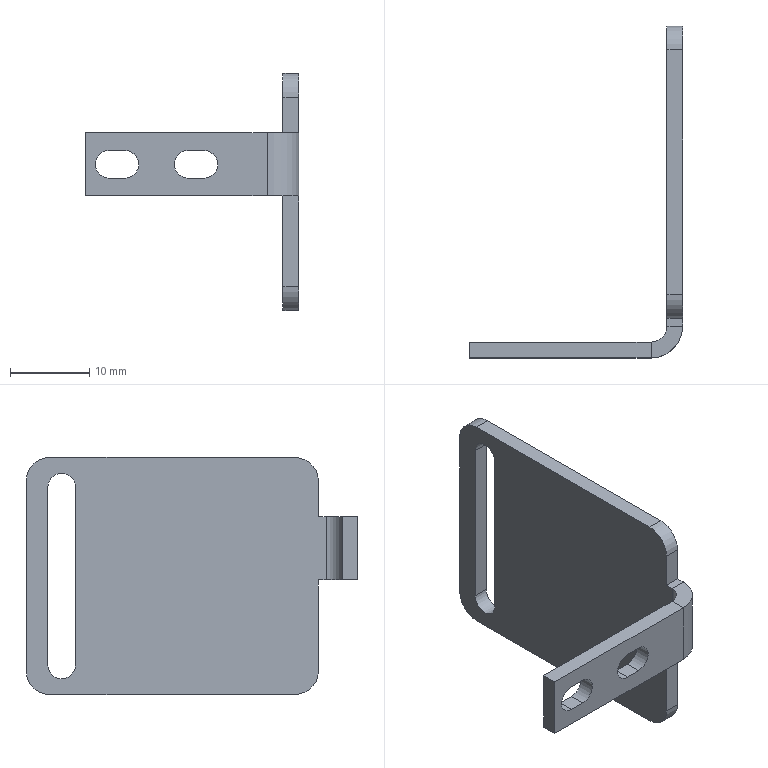Part | STEP file | Cup gripper lift proximity switch bracket 02V1.201001 | 1 solid | 37 faces | box 27 x 42 x 30 mm | volume 2421 mm3 | plane 22 | cylinder 15 | commonest cylinder face diameters 3.5 x9 6 x4 4 x1 8 x1